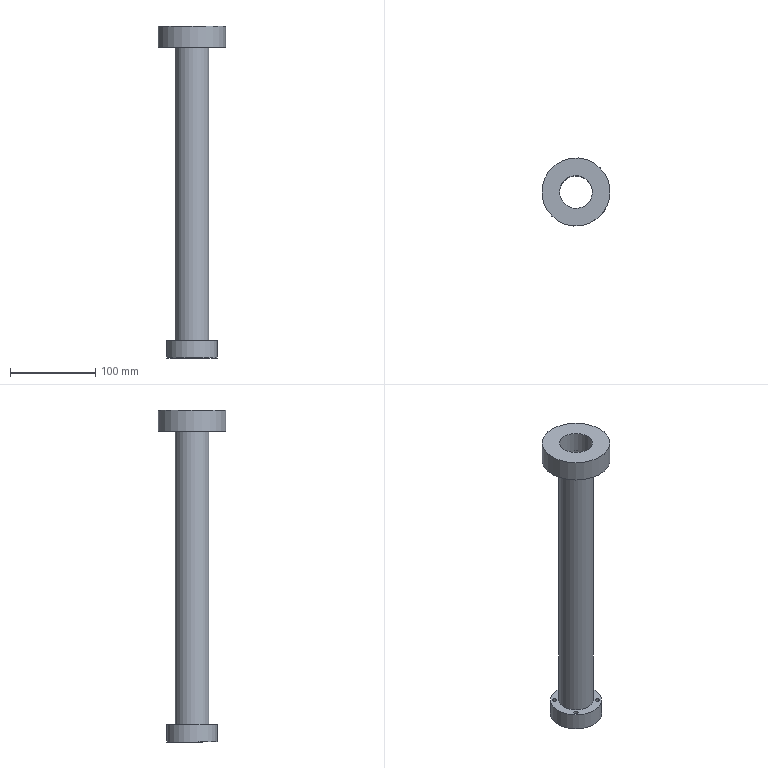Part | STEP file | Q6.0 _6_ diameter hole 1_id554_x_t | 1 solid | 12 faces | box 80 x 80 x 390 mm | volume 160160 mm3 | cylinder 8 | plane 4 | commonest cylinder face diameters 5 x4 38.5 x1 40 x1 60 x1 80 x1
STEP:
#1=CARTESIAN_POINT('',(1605.858,-185.858,20.));
#2=VERTEX_POINT('',#1);
#3=CARTESIAN_POINT('',(1620.,-200.,20.));
#4=DIRECTION('',(0.,0.,-1.));
#5=DIRECTION('',(-0.7071,0.7071,0.));
#6=AXIS2_PLACEMENT_3D('',#3,#4,#5);
#7=CIRCLE('',#6,20.);
#8=EDGE_CURVE('',#2,#2,#7,.T.);
#9=ORIENTED_EDGE('',*,*,#8,.F.);
#10=EDGE_LOOP('',(#9));
#11=FACE_BOUND('',#10,.T.);
#12=CARTESIAN_POINT('',(1605.858,-185.858,365.));
#13=VERTEX_POINT('',#12);
#14=CARTESIAN_POINT('',(1620.,-200.,365.));
#15=DIRECTION('',(0.,0.,-1.));
#16=DIRECTION('',(-0.7071,0.7071,0.));
#17=AXIS2_PLACEMENT_3D('',#14,#15,#16);
#18=CIRCLE('',#17,20.);
#19=EDGE_CURVE('',#13,#13,#18,.T.);
#20=ORIENTED_EDGE('',*,*,#19,.T.);
#21=EDGE_LOOP('',(#20));
#22=FACE_BOUND('',#21,.T.);
#23=CARTESIAN_POINT('',(1620.,-200.,15.));
#24=DIRECTION('',(0.,0.,1.));
#25=DIRECTION('',(0.7071,0.7071,0.));
#26=AXIS2_PLACEMENT_3D('',#23,#24,#25);
#27=CYLINDRICAL_SURFACE('',#26,20.);
#28=ADVANCED_FACE('',(#11,#22),#27,.T.);
#29=CARTESIAN_POINT('',(1598.787,-178.787,20.));
#30=VERTEX_POINT('',#29);
#31=CARTESIAN_POINT('',(1620.,-200.,20.));
#32=DIRECTION('',(0.,0.,-1.));
#33=DIRECTION('',(-0.7071,0.7071,0.));
#34=AXIS2_PLACEMENT_3D('',#31,#32,#33);
#35=CIRCLE('',#34,30.);
#36=EDGE_CURVE('',#30,#30,#35,.T.);
#37=ORIENTED_EDGE('',*,*,#36,.T.);
#38=EDGE_LOOP('',(#37));
#39=FACE_BOUND('',#38,.T.);
#40=CARTESIAN_POINT('',(1598.787,-178.787,0.));
#41=VERTEX_POINT('',#40);
#42=CARTESIAN_POINT('',(1620.,-200.,0.));
#43=DIRECTION('',(0.,0.,-1.));
#44=DIRECTION('',(-0.7071,0.7071,0.));
#45=AXIS2_PLACEMENT_3D('',#42,#43,#44);
#46=CIRCLE('',#45,30.);
#47=EDGE_CURVE('',#41,#41,#46,.T.);
#48=ORIENTED_EDGE('',*,*,#47,.F.);
#49=EDGE_LOOP('',(#48));
#50=FACE_BOUND('',#49,.T.);
#51=CARTESIAN_POINT('',(1620.,-200.,0.));
#52=DIRECTION('',(0.,0.,1.));
#53=DIRECTION('',(0.7071,0.7071,0.));
#54=AXIS2_PLACEMENT_3D('',#51,#52,#53);
#55=CYLINDRICAL_SURFACE('',#54,30.);
#56=ADVANCED_FACE('',(#39,#50),#55,.T.);
#57=CARTESIAN_POINT('',(1648.284,-171.716,365.));
#58=VERTEX_POINT('',#57);
#59=CARTESIAN_POINT('',(1620.,-200.,365.));
#60=DIRECTION('',(0.,0.,-1.));
#61=DIRECTION('',(0.7071,0.7071,0.));
#62=AXIS2_PLACEMENT_3D('',#59,#60,#61);
#63=CIRCLE('',#62,40.);
#64=EDGE_CURVE('',#58,#58,#63,.T.);
#65=ORIENTED_EDGE('',*,*,#64,.T.);
#66=EDGE_LOOP('',(#65));
#67=FACE_BOUND('',#66,.T.);
#68=ORIENTED_EDGE('',*,*,#19,.F.);
#69=EDGE_LOOP('',(#68));
#70=FACE_BOUND('',#69,.T.);
#71=CARTESIAN_POINT('',(1620.,-200.,365.));
#72=DIRECTION('',(0.,0.,-1.));
#73=DIRECTION('',(-0.7071,-0.7071,0.));
#74=AXIS2_PLACEMENT_3D('',#71,#72,#73);
#75=PLANE('',#74);
#76=ADVANCED_FACE('',(#67,#70),#75,.T.);
#77=CARTESIAN_POINT('',(1591.716,-228.284,390.));
#78=VERTEX_POINT('',#77);
#79=CARTESIAN_POINT('',(1620.,-200.,390.));
#80=DIRECTION('',(0.,0.,-1.));
#81=DIRECTION('',(-0.7071,-0.7071,0.));
#82=AXIS2_PLACEMENT_3D('',#79,#80,#81);
#83=CIRCLE('',#82,40.);
#84=EDGE_CURVE('',#78,#78,#83,.T.);
#85=ORIENTED_EDGE('',*,*,#84,.T.);
#86=EDGE_LOOP('',(#85));
#87=FACE_BOUND('',#86,.T.);
#88=ORIENTED_EDGE('',*,*,#64,.F.);
#89=EDGE_LOOP('',(#88));
#90=FACE_BOUND('',#89,.T.);
#91=CARTESIAN_POINT('',(1620.,-200.,365.));
#92=DIRECTION('',(0.,0.,1.));
#93=DIRECTION('',(0.7071,0.7071,0.));
#94=AXIS2_PLACEMENT_3D('',#91,#92,#93);
#95=CYLINDRICAL_SURFACE('',#94,40.);
#96=ADVANCED_FACE('',(#87,#90),#95,.T.);
#97=CARTESIAN_POINT('',(1600.555,-215.91,20.));
#98=VERTEX_POINT('',#97);
#99=CARTESIAN_POINT('',(1602.322,-217.678,20.));
#100=DIRECTION('',(0.,0.,1.));
#101=DIRECTION('',(-0.7071,0.7071,0.));
#102=AXIS2_PLACEMENT_3D('',#99,#100,#101);
#103=CIRCLE('',#102,2.5);
#104=EDGE_CURVE('',#98,#98,#103,.T.);
#105=ORIENTED_EDGE('',*,*,#104,.F.);
#106=EDGE_LOOP('',(#105));
#107=FACE_BOUND('',#106,.T.);
#108=CARTESIAN_POINT('',(1635.91,-215.91,20.));
#109=VERTEX_POINT('',#108);
#110=CARTESIAN_POINT('',(1637.678,-217.678,20.));
#111=DIRECTION('',(0.,0.,1.));
#112=DIRECTION('',(-0.7071,0.7071,0.));
#113=AXIS2_PLACEMENT_3D('',#110,#111,#112);
#114=CIRCLE('',#113,2.5);
#115=EDGE_CURVE('',#109,#109,#114,.T.);
#116=ORIENTED_EDGE('',*,*,#115,.F.);
#117=EDGE_LOOP('',(#116));
#118=FACE_BOUND('',#117,.T.);
#119=CARTESIAN_POINT('',(1635.91,-180.555,20.));
#120=VERTEX_POINT('',#119);
#121=CARTESIAN_POINT('',(1637.678,-182.322,20.));
#122=DIRECTION('',(0.,0.,1.));
#123=DIRECTION('',(-0.7071,0.7071,0.));
#124=AXIS2_PLACEMENT_3D('',#121,#122,#123);
#125=CIRCLE('',#124,2.5);
#126=EDGE_CURVE('',#120,#120,#125,.T.);
#127=ORIENTED_EDGE('',*,*,#126,.F.);
#128=EDGE_LOOP('',(#127));
#129=FACE_BOUND('',#128,.T.);
#130=ORIENTED_EDGE('',*,*,#8,.T.);
#131=EDGE_LOOP('',(#130));
#132=FACE_BOUND('',#131,.T.);
#133=CARTESIAN_POINT('',(1600.555,-180.555,20.));
#134=VERTEX_POINT('',#133);
#135=CARTESIAN_POINT('',(1602.322,-182.322,20.));
#136=DIRECTION('',(0.,0.,1.));
#137=DIRECTION('',(-0.7071,0.7071,0.));
#138=AXIS2_PLACEMENT_3D('',#135,#136,#137);
#139=CIRCLE('',#138,2.5);
#140=EDGE_CURVE('',#134,#134,#139,.T.);
#141=ORIENTED_EDGE('',*,*,#140,.F.);
#142=EDGE_LOOP('',(#141));
#143=FACE_BOUND('',#142,.T.);
#144=ORIENTED_EDGE('',*,*,#36,.F.);
#145=EDGE_LOOP('',(#144));
#146=FACE_BOUND('',#145,.T.);
#147=CARTESIAN_POINT('',(1620.,-200.,20.));
#148=DIRECTION('',(0.,0.,-1.));
#149=DIRECTION('',(-0.7071,-0.7071,0.));
#150=AXIS2_PLACEMENT_3D('',#147,#148,#149);
#151=PLANE('',#150);
#152=ADVANCED_FACE('',(#107,#118,#129,#132,#143,#146),#151,.F.);
#153=CARTESIAN_POINT('',(1600.555,-180.555,0.));
#154=VERTEX_POINT('',#153);
#155=CARTESIAN_POINT('',(1602.322,-182.322,0.));
#156=DIRECTION('',(0.,0.,1.));
#157=DIRECTION('',(-0.7071,0.7071,0.));
#158=AXIS2_PLACEMENT_3D('',#155,#156,#157);
#159=CIRCLE('',#158,2.5);
#160=EDGE_CURVE('',#154,#154,#159,.T.);
#161=ORIENTED_EDGE('',*,*,#160,.T.);
#162=EDGE_LOOP('',(#161));
#163=FACE_BOUND('',#162,.T.);
#164=CARTESIAN_POINT('',(1600.555,-215.91,0.));
#165=VERTEX_POINT('',#164);
#166=CARTESIAN_POINT('',(1602.322,-217.678,0.));
#167=DIRECTION('',(0.,0.,1.));
#168=DIRECTION('',(-0.7071,0.7071,0.));
#169=AXIS2_PLACEMENT_3D('',#166,#167,#168);
#170=CIRCLE('',#169,2.5);
#171=EDGE_CURVE('',#165,#165,#170,.T.);
#172=ORIENTED_EDGE('',*,*,#171,.T.);
#173=EDGE_LOOP('',(#172));
#174=FACE_BOUND('',#173,.T.);
#175=CARTESIAN_POINT('',(1635.91,-215.91,0.));
#176=VERTEX_POINT('',#175);
#177=CARTESIAN_POINT('',(1637.678,-217.678,0.));
#178=DIRECTION('',(0.,0.,1.));
#179=DIRECTION('',(-0.7071,0.7071,0.));
#180=AXIS2_PLACEMENT_3D('',#177,#178,#179);
#181=CIRCLE('',#180,2.5);
#182=EDGE_CURVE('',#176,#176,#181,.T.);
#183=ORIENTED_EDGE('',*,*,#182,.T.);
#184=EDGE_LOOP('',(#183));
#185=FACE_BOUND('',#184,.T.);
#186=CARTESIAN_POINT('',(1635.91,-180.555,0.));
#187=VERTEX_POINT('',#186);
#188=CARTESIAN_POINT('',(1637.678,-182.322,0.));
#189=DIRECTION('',(0.,0.,1.));
#190=DIRECTION('',(-0.7071,0.7071,0.));
#191=AXIS2_PLACEMENT_3D('',#188,#189,#190);
#192=CIRCLE('',#191,2.5);
#193=EDGE_CURVE('',#187,#187,#192,.T.);
#194=ORIENTED_EDGE('',*,*,#193,.T.);
#195=EDGE_LOOP('',(#194));
#196=FACE_BOUND('',#195,.T.);
#197=ORIENTED_EDGE('',*,*,#47,.T.);
#198=EDGE_LOOP('',(#197));
#199=FACE_BOUND('',#198,.T.);
#200=CARTESIAN_POINT('',(1606.388,-186.388,0.));
#201=VERTEX_POINT('',#200);
#202=CARTESIAN_POINT('',(1620.,-200.,0.));
#203=DIRECTION('',(0.,0.,-1.));
#204=DIRECTION('',(-0.7071,0.7071,0.));
#205=AXIS2_PLACEMENT_3D('',#202,#203,#204);
#206=CIRCLE('',#205,19.25);
#207=EDGE_CURVE('',#201,#201,#206,.T.);
#208=ORIENTED_EDGE('',*,*,#207,.F.);
#209=EDGE_LOOP('',(#208));
#210=FACE_BOUND('',#209,.T.);
#211=CARTESIAN_POINT('',(1620.,-200.,0.));
#212=DIRECTION('',(0.,0.,-1.));
#213=DIRECTION('',(-0.7071,-0.7071,0.));
#214=AXIS2_PLACEMENT_3D('',#211,#212,#213);
#215=PLANE('',#214);
#216=ADVANCED_FACE('',(#163,#174,#185,#196,#199,#210),#215,.T.);
#217=CARTESIAN_POINT('',(1606.388,-186.388,390.));
#218=VERTEX_POINT('',#217);
#219=CARTESIAN_POINT('',(1620.,-200.,390.));
#220=DIRECTION('',(0.,0.,-1.));
#221=DIRECTION('',(-0.7071,0.7071,0.));
#222=AXIS2_PLACEMENT_3D('',#219,#220,#221);
#223=CIRCLE('',#222,19.25);
#224=EDGE_CURVE('',#218,#218,#223,.T.);
#225=ORIENTED_EDGE('',*,*,#224,.F.);
#226=EDGE_LOOP('',(#225));
#227=FACE_BOUND('',#226,.T.);
#228=ORIENTED_EDGE('',*,*,#207,.T.);
#229=EDGE_LOOP('',(#228));
#230=FACE_BOUND('',#229,.T.);
#231=CARTESIAN_POINT('',(1620.,-200.,453.64));
#232=DIRECTION('',(0.,0.,-1.));
#233=DIRECTION('',(-0.7071,-0.7071,0.));
#234=AXIS2_PLACEMENT_3D('',#231,#232,#233);
#235=CYLINDRICAL_SURFACE('',#234,19.25);
#236=ADVANCED_FACE('',(#227,#230),#235,.F.);
#237=ORIENTED_EDGE('',*,*,#84,.F.);
#238=EDGE_LOOP('',(#237));
#239=FACE_BOUND('',#238,.T.);
#240=ORIENTED_EDGE('',*,*,#224,.T.);
#241=EDGE_LOOP('',(#240));
#242=FACE_BOUND('',#241,.T.);
#243=CARTESIAN_POINT('',(1620.,-200.,390.));
#244=DIRECTION('',(0.,0.,-1.));
#245=DIRECTION('',(-0.7071,-0.7071,0.));
#246=AXIS2_PLACEMENT_3D('',#243,#244,#245);
#247=PLANE('',#246);
#248=ADVANCED_FACE('',(#239,#242),#247,.F.);
#249=ORIENTED_EDGE('',*,*,#126,.T.);
#250=EDGE_LOOP('',(#249));
#251=FACE_BOUND('',#250,.T.);
#252=ORIENTED_EDGE('',*,*,#193,.F.);
#253=EDGE_LOOP('',(#252));
#254=FACE_BOUND('',#253,.T.);
#255=CARTESIAN_POINT('',(1637.678,-182.322,-1.));
#256=DIRECTION('',(0.,0.,1.));
#257=DIRECTION('',(0.7071,0.7071,0.));
#258=AXIS2_PLACEMENT_3D('',#255,#256,#257);
#259=CYLINDRICAL_SURFACE('',#258,2.5);
#260=ADVANCED_FACE('',(#251,#254),#259,.F.);
#261=ORIENTED_EDGE('',*,*,#115,.T.);
#262=EDGE_LOOP('',(#261));
#263=FACE_BOUND('',#262,.T.);
#264=ORIENTED_EDGE('',*,*,#182,.F.);
#265=EDGE_LOOP('',(#264));
#266=FACE_BOUND('',#265,.T.);
#267=CARTESIAN_POINT('',(1637.678,-217.678,-1.));
#268=DIRECTION('',(0.,0.,1.));
#269=DIRECTION('',(0.7071,0.7071,0.));
#270=AXIS2_PLACEMENT_3D('',#267,#268,#269);
#271=CYLINDRICAL_SURFACE('',#270,2.5);
#272=ADVANCED_FACE('',(#263,#266),#271,.F.);
#273=ORIENTED_EDGE('',*,*,#104,.T.);
#274=EDGE_LOOP('',(#273));
#275=FACE_BOUND('',#274,.T.);
#276=ORIENTED_EDGE('',*,*,#171,.F.);
#277=EDGE_LOOP('',(#276));
#278=FACE_BOUND('',#277,.T.);
#279=CARTESIAN_POINT('',(1602.322,-217.678,-1.));
#280=DIRECTION('',(0.,0.,1.));
#281=DIRECTION('',(0.7071,0.7071,0.));
#282=AXIS2_PLACEMENT_3D('',#279,#280,#281);
#283=CYLINDRICAL_SURFACE('',#282,2.5);
#284=ADVANCED_FACE('',(#275,#278),#283,.F.);
#285=ORIENTED_EDGE('',*,*,#140,.T.);
#286=EDGE_LOOP('',(#285));
#287=FACE_BOUND('',#286,.T.);
#288=ORIENTED_EDGE('',*,*,#160,.F.);
#289=EDGE_LOOP('',(#288));
#290=FACE_BOUND('',#289,.T.);
#291=CARTESIAN_POINT('',(1602.322,-182.322,-1.));
#292=DIRECTION('',(0.,0.,1.));
#293=DIRECTION('',(0.7071,0.7071,0.));
#294=AXIS2_PLACEMENT_3D('',#291,#292,#293);
#295=CYLINDRICAL_SURFACE('',#294,2.5);
#296=ADVANCED_FACE('',(#287,#290),#295,.F.);
#297=CLOSED_SHELL('',(#28,#56,#76,#96,#152,#216,#236,#248,#260,#272,#284,#296));
#298=MANIFOLD_SOLID_BREP('',#297);
#299=(LENGTH_UNIT()NAMED_UNIT(*)SI_UNIT(.MILLI.,.METRE.));
#300=UNCERTAINTY_MEASURE_WITH_UNIT(LENGTH_MEASURE(0.00002),#299,'','');
#301=(NAMED_UNIT(*)PLANE_ANGLE_UNIT()SI_UNIT($,.RADIAN.));
#302=PLANE_ANGLE_MEASURE_WITH_UNIT(PLANE_ANGLE_MEASURE(0.01745),#301);
#303=DIMENSIONAL_EXPONENTS(0.,0.,0.,0.,0.,0.,0.);
#304=(CONVERSION_BASED_UNIT('DEGREE',#302)NAMED_UNIT(#303)PLANE_ANGLE_UNIT());
#305=(NAMED_UNIT(*)SI_UNIT($,.STERADIAN.)SOLID_ANGLE_UNIT());
#306=(GEOMETRIC_REPRESENTATION_CONTEXT(3)GLOBAL_UNCERTAINTY_ASSIGNED_CONTEXT((#300))GLOBAL_UNIT_ASSIGNED_CONTEXT((#299,#304,#305))REPRESENTATION_CONTEXT('',''));
#307=ADVANCED_BREP_SHAPE_REPRESENTATION('',(#298),#306);